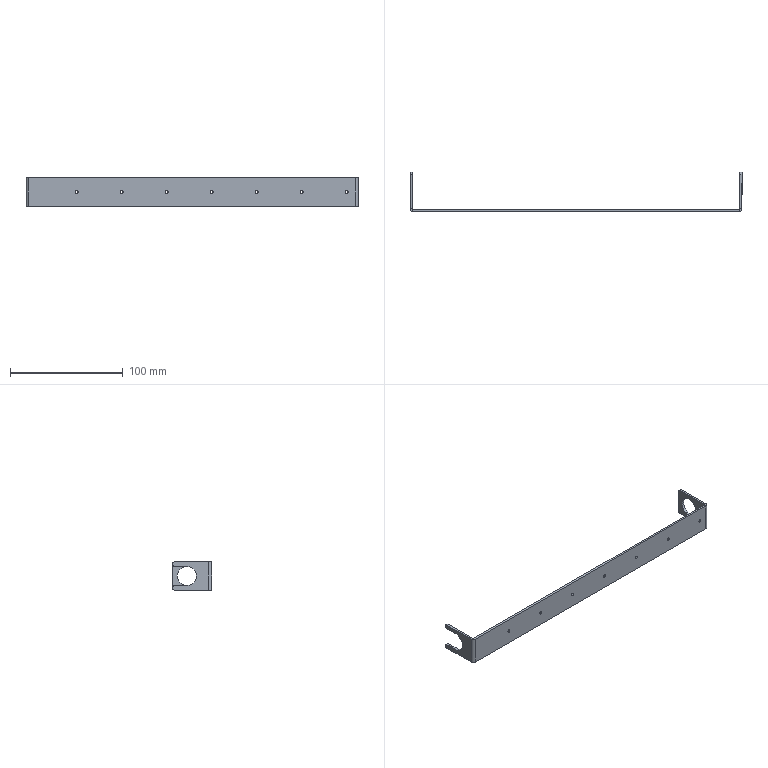Part | SolidWorks | features HoleWzd 2, ICE 2, EdgeFlange 1, Fillet 1, FlatPattern 1, LPattern 1, SMBaseFlange 1, SheetMetal 1 | 1 solid | 47 faces | box 295 x 35 x 25 mm | volume 16784 mm3 | cylinder 28 | plane 19 | commonest cylinder face diameters 2.5 x14 4 x6 17 x4 1 x2 5 x2
STEP:
#1=CARTESIAN_POINT('',(97.5,-2.,-1.25));
#2=VERTEX_POINT('',#1);
#3=CARTESIAN_POINT('',(97.5,-2.,1.25));
#4=VERTEX_POINT('',#3);
#5=CARTESIAN_POINT('',(97.5,-2.,0.));
#6=DIRECTION('',(0.,1.,0.));
#7=DIRECTION('',(0.,0.,1.));
#8=AXIS2_PLACEMENT_3D('',#5,#6,#7);
#9=CIRCLE('',#8,1.25);
#10=EDGE_CURVE('',#2,#4,#9,.T.);
#11=ORIENTED_EDGE('',*,*,#10,.F.);
#12=CARTESIAN_POINT('',(97.5,0.,-1.25));
#13=VERTEX_POINT('',#12);
#14=CARTESIAN_POINT('',(97.5,0.,-1.25));
#15=DIRECTION('',(0.,1.,0.));
#16=VECTOR('',#15,1000.);
#17=LINE('',#14,#16);
#18=EDGE_CURVE('',#2,#13,#17,.T.);
#19=ORIENTED_EDGE('',*,*,#18,.T.);
#20=CARTESIAN_POINT('',(97.5,0.,1.25));
#21=VERTEX_POINT('',#20);
#22=CARTESIAN_POINT('',(97.5,0.,0.));
#23=DIRECTION('',(0.,1.,0.));
#24=DIRECTION('',(0.,0.,1.));
#25=AXIS2_PLACEMENT_3D('',#22,#23,#24);
#26=CIRCLE('',#25,1.25);
#27=EDGE_CURVE('',#13,#21,#26,.T.);
#28=ORIENTED_EDGE('',*,*,#27,.T.);
#29=CARTESIAN_POINT('',(97.5,0.,1.25));
#30=DIRECTION('',(0.,1.,0.));
#31=VECTOR('',#30,1000.);
#32=LINE('',#29,#31);
#33=EDGE_CURVE('',#4,#21,#32,.T.);
#34=ORIENTED_EDGE('',*,*,#33,.F.);
#35=EDGE_LOOP('',(#11,#19,#28,#34));
#36=FACE_OUTER_BOUND('',#35,.T.);
#37=CARTESIAN_POINT('',(97.5,0.,0.));
#38=DIRECTION('',(0.,1.,0.));
#39=DIRECTION('',(0.,0.,1.));
#40=AXIS2_PLACEMENT_3D('',#37,#38,#39);
#41=CYLINDRICAL_SURFACE('',#40,1.25);
#42=ADVANCED_FACE('',(#36),#41,.F.);
#43=CARTESIAN_POINT('',(137.5,-2.,-1.25));
#44=VERTEX_POINT('',#43);
#45=CARTESIAN_POINT('',(137.5,-2.,1.25));
#46=VERTEX_POINT('',#45);
#47=CARTESIAN_POINT('',(137.5,-2.,0.));
#48=DIRECTION('',(0.,1.,0.));
#49=DIRECTION('',(0.,0.,1.));
#50=AXIS2_PLACEMENT_3D('',#47,#48,#49);
#51=CIRCLE('',#50,1.25);
#52=EDGE_CURVE('',#44,#46,#51,.T.);
#53=ORIENTED_EDGE('',*,*,#52,.F.);
#54=CARTESIAN_POINT('',(137.5,0.,-1.25));
#55=VERTEX_POINT('',#54);
#56=CARTESIAN_POINT('',(137.5,0.,-1.25));
#57=DIRECTION('',(0.,1.,0.));
#58=VECTOR('',#57,1000.);
#59=LINE('',#56,#58);
#60=EDGE_CURVE('',#44,#55,#59,.T.);
#61=ORIENTED_EDGE('',*,*,#60,.T.);
#62=CARTESIAN_POINT('',(137.5,0.,1.25));
#63=VERTEX_POINT('',#62);
#64=CARTESIAN_POINT('',(137.5,0.,0.));
#65=DIRECTION('',(0.,1.,0.));
#66=DIRECTION('',(0.,0.,1.));
#67=AXIS2_PLACEMENT_3D('',#64,#65,#66);
#68=CIRCLE('',#67,1.25);
#69=EDGE_CURVE('',#55,#63,#68,.T.);
#70=ORIENTED_EDGE('',*,*,#69,.T.);
#71=CARTESIAN_POINT('',(137.5,0.,1.25));
#72=DIRECTION('',(0.,1.,0.));
#73=VECTOR('',#72,1000.);
#74=LINE('',#71,#73);
#75=EDGE_CURVE('',#46,#63,#74,.T.);
#76=ORIENTED_EDGE('',*,*,#75,.F.);
#77=EDGE_LOOP('',(#53,#61,#70,#76));
#78=FACE_OUTER_BOUND('',#77,.T.);
#79=CARTESIAN_POINT('',(137.5,0.,0.));
#80=DIRECTION('',(0.,1.,0.));
#81=DIRECTION('',(0.,0.,1.));
#82=AXIS2_PLACEMENT_3D('',#79,#80,#81);
#83=CYLINDRICAL_SURFACE('',#82,1.25);
#84=ADVANCED_FACE('',(#78),#83,.F.);
#85=CARTESIAN_POINT('',(-145.5,20.,8.5));
#86=VERTEX_POINT('',#85);
#87=CARTESIAN_POINT('',(-145.5,11.5,0.));
#88=VERTEX_POINT('',#87);
#89=CARTESIAN_POINT('',(-145.5,20.,0.));
#90=DIRECTION('',(1.,0.,0.));
#91=DIRECTION('',(0.,1.,0.));
#92=AXIS2_PLACEMENT_3D('',#89,#90,#91);
#93=CIRCLE('',#92,8.5);
#94=EDGE_CURVE('',#86,#88,#93,.T.);
#95=ORIENTED_EDGE('',*,*,#94,.T.);
#96=CARTESIAN_POINT('',(-147.5,11.5,0.));
#97=VERTEX_POINT('',#96);
#98=CARTESIAN_POINT('',(-137.5,11.5,0.));
#99=DIRECTION('',(-1.,0.,0.));
#100=VECTOR('',#99,1000.);
#101=LINE('',#98,#100);
#102=EDGE_CURVE('',#88,#97,#101,.T.);
#103=ORIENTED_EDGE('',*,*,#102,.T.);
#104=CARTESIAN_POINT('',(-147.5,20.,8.5));
#105=VERTEX_POINT('',#104);
#106=CARTESIAN_POINT('',(-147.5,20.,0.));
#107=DIRECTION('',(-1.,0.,0.));
#108=DIRECTION('',(0.,-1.,0.));
#109=AXIS2_PLACEMENT_3D('',#106,#107,#108);
#110=CIRCLE('',#109,8.5);
#111=EDGE_CURVE('',#97,#105,#110,.T.);
#112=ORIENTED_EDGE('',*,*,#111,.T.);
#113=CARTESIAN_POINT('',(-137.5,20.,8.5));
#114=DIRECTION('',(-1.,0.,0.));
#115=VECTOR('',#114,1000.);
#116=LINE('',#113,#115);
#117=EDGE_CURVE('',#86,#105,#116,.T.);
#118=ORIENTED_EDGE('',*,*,#117,.F.);
#119=EDGE_LOOP('',(#95,#103,#112,#118));
#120=FACE_OUTER_BOUND('',#119,.T.);
#121=CARTESIAN_POINT('',(-137.5,20.,0.));
#122=DIRECTION('',(-1.,0.,0.));
#123=DIRECTION('',(0.,-1.,0.));
#124=AXIS2_PLACEMENT_3D('',#121,#122,#123);
#125=CYLINDRICAL_SURFACE('',#124,8.5);
#126=ADVANCED_FACE('',(#120),#125,.F.);
#127=CARTESIAN_POINT('',(145.5,28.5,0.));
#128=VERTEX_POINT('',#127);
#129=CARTESIAN_POINT('',(145.5,11.5,0.));
#130=VERTEX_POINT('',#129);
#131=CARTESIAN_POINT('',(145.5,20.,0.));
#132=DIRECTION('',(-1.,0.,0.));
#133=DIRECTION('',(0.,-1.,0.));
#134=AXIS2_PLACEMENT_3D('',#131,#132,#133);
#135=CIRCLE('',#134,8.5);
#136=EDGE_CURVE('',#128,#130,#135,.T.);
#137=ORIENTED_EDGE('',*,*,#136,.T.);
#138=CARTESIAN_POINT('',(147.5,11.5,0.));
#139=VERTEX_POINT('',#138);
#140=CARTESIAN_POINT('',(137.5,11.5,0.));
#141=DIRECTION('',(1.,0.,0.));
#142=VECTOR('',#141,1000.);
#143=LINE('',#140,#142);
#144=EDGE_CURVE('',#130,#139,#143,.T.);
#145=ORIENTED_EDGE('',*,*,#144,.T.);
#146=CARTESIAN_POINT('',(147.5,28.5,0.));
#147=VERTEX_POINT('',#146);
#148=CARTESIAN_POINT('',(147.5,20.,0.));
#149=DIRECTION('',(1.,0.,0.));
#150=DIRECTION('',(0.,1.,0.));
#151=AXIS2_PLACEMENT_3D('',#148,#149,#150);
#152=CIRCLE('',#151,8.5);
#153=EDGE_CURVE('',#139,#147,#152,.T.);
#154=ORIENTED_EDGE('',*,*,#153,.T.);
#155=CARTESIAN_POINT('',(137.5,28.5,0.));
#156=DIRECTION('',(1.,0.,0.));
#157=VECTOR('',#156,1000.);
#158=LINE('',#155,#157);
#159=EDGE_CURVE('',#128,#147,#158,.T.);
#160=ORIENTED_EDGE('',*,*,#159,.F.);
#161=EDGE_LOOP('',(#137,#145,#154,#160));
#162=FACE_OUTER_BOUND('',#161,.T.);
#163=CARTESIAN_POINT('',(137.5,20.,0.));
#164=DIRECTION('',(1.,0.,0.));
#165=DIRECTION('',(0.,1.,0.));
#166=AXIS2_PLACEMENT_3D('',#163,#164,#165);
#167=CYLINDRICAL_SURFACE('',#166,8.5);
#168=ADVANCED_FACE('',(#162),#167,.F.);
#169=CARTESIAN_POINT('',(57.5,-2.,-1.25));
#170=VERTEX_POINT('',#169);
#171=CARTESIAN_POINT('',(57.5,-2.,1.25));
#172=VERTEX_POINT('',#171);
#173=CARTESIAN_POINT('',(57.5,-2.,0.));
#174=DIRECTION('',(0.,1.,0.));
#175=DIRECTION('',(0.,0.,1.));
#176=AXIS2_PLACEMENT_3D('',#173,#174,#175);
#177=CIRCLE('',#176,1.25);
#178=EDGE_CURVE('',#170,#172,#177,.T.);
#179=ORIENTED_EDGE('',*,*,#178,.F.);
#180=CARTESIAN_POINT('',(57.5,0.,-1.25));
#181=VERTEX_POINT('',#180);
#182=CARTESIAN_POINT('',(57.5,0.,-1.25));
#183=DIRECTION('',(0.,1.,0.));
#184=VECTOR('',#183,1000.);
#185=LINE('',#182,#184);
#186=EDGE_CURVE('',#170,#181,#185,.T.);
#187=ORIENTED_EDGE('',*,*,#186,.T.);
#188=CARTESIAN_POINT('',(57.5,0.,1.25));
#189=VERTEX_POINT('',#188);
#190=CARTESIAN_POINT('',(57.5,0.,0.));
#191=DIRECTION('',(0.,1.,0.));
#192=DIRECTION('',(0.,0.,1.));
#193=AXIS2_PLACEMENT_3D('',#190,#191,#192);
#194=CIRCLE('',#193,1.25);
#195=EDGE_CURVE('',#181,#189,#194,.T.);
#196=ORIENTED_EDGE('',*,*,#195,.T.);
#197=CARTESIAN_POINT('',(57.5,0.,1.25));
#198=DIRECTION('',(0.,1.,0.));
#199=VECTOR('',#198,1000.);
#200=LINE('',#197,#199);
#201=EDGE_CURVE('',#172,#189,#200,.T.);
#202=ORIENTED_EDGE('',*,*,#201,.F.);
#203=EDGE_LOOP('',(#179,#187,#196,#202));
#204=FACE_OUTER_BOUND('',#203,.T.);
#205=CARTESIAN_POINT('',(57.5,0.,0.));
#206=DIRECTION('',(0.,1.,0.));
#207=DIRECTION('',(0.,0.,1.));
#208=AXIS2_PLACEMENT_3D('',#205,#206,#207);
#209=CYLINDRICAL_SURFACE('',#208,1.25);
#210=ADVANCED_FACE('',(#204),#209,.F.);
#211=CARTESIAN_POINT('',(17.5,-2.,-1.25));
#212=VERTEX_POINT('',#211);
#213=CARTESIAN_POINT('',(17.5,-2.,1.25));
#214=VERTEX_POINT('',#213);
#215=CARTESIAN_POINT('',(17.5,-2.,0.));
#216=DIRECTION('',(0.,1.,0.));
#217=DIRECTION('',(0.,0.,1.));
#218=AXIS2_PLACEMENT_3D('',#215,#216,#217);
#219=CIRCLE('',#218,1.25);
#220=EDGE_CURVE('',#212,#214,#219,.T.);
#221=ORIENTED_EDGE('',*,*,#220,.F.);
#222=CARTESIAN_POINT('',(17.5,0.,-1.25));
#223=VERTEX_POINT('',#222);
#224=CARTESIAN_POINT('',(17.5,0.,-1.25));
#225=DIRECTION('',(0.,1.,0.));
#226=VECTOR('',#225,1000.);
#227=LINE('',#224,#226);
#228=EDGE_CURVE('',#212,#223,#227,.T.);
#229=ORIENTED_EDGE('',*,*,#228,.T.);
#230=CARTESIAN_POINT('',(17.5,0.,1.25));
#231=VERTEX_POINT('',#230);
#232=CARTESIAN_POINT('',(17.5,0.,0.));
#233=DIRECTION('',(0.,1.,0.));
#234=DIRECTION('',(0.,0.,1.));
#235=AXIS2_PLACEMENT_3D('',#232,#233,#234);
#236=CIRCLE('',#235,1.25);
#237=EDGE_CURVE('',#223,#231,#236,.T.);
#238=ORIENTED_EDGE('',*,*,#237,.T.);
#239=CARTESIAN_POINT('',(17.5,0.,1.25));
#240=DIRECTION('',(0.,1.,0.));
#241=VECTOR('',#240,1000.);
#242=LINE('',#239,#241);
#243=EDGE_CURVE('',#214,#231,#242,.T.);
#244=ORIENTED_EDGE('',*,*,#243,.F.);
#245=EDGE_LOOP('',(#221,#229,#238,#244));
#246=FACE_OUTER_BOUND('',#245,.T.);
#247=CARTESIAN_POINT('',(17.5,0.,0.));
#248=DIRECTION('',(0.,1.,0.));
#249=DIRECTION('',(0.,0.,1.));
#250=AXIS2_PLACEMENT_3D('',#247,#248,#249);
#251=CYLINDRICAL_SURFACE('',#250,1.25);
#252=ADVANCED_FACE('',(#246),#251,.F.);
#253=CARTESIAN_POINT('',(-22.5,-2.,-1.25));
#254=VERTEX_POINT('',#253);
#255=CARTESIAN_POINT('',(-22.5,-2.,1.25));
#256=VERTEX_POINT('',#255);
#257=CARTESIAN_POINT('',(-22.5,-2.,0.));
#258=DIRECTION('',(0.,1.,0.));
#259=DIRECTION('',(0.,0.,1.));
#260=AXIS2_PLACEMENT_3D('',#257,#258,#259);
#261=CIRCLE('',#260,1.25);
#262=EDGE_CURVE('',#254,#256,#261,.T.);
#263=ORIENTED_EDGE('',*,*,#262,.F.);
#264=CARTESIAN_POINT('',(-22.5,0.,-1.25));
#265=VERTEX_POINT('',#264);
#266=CARTESIAN_POINT('',(-22.5,0.,-1.25));
#267=DIRECTION('',(0.,1.,0.));
#268=VECTOR('',#267,1000.);
#269=LINE('',#266,#268);
#270=EDGE_CURVE('',#254,#265,#269,.T.);
#271=ORIENTED_EDGE('',*,*,#270,.T.);
#272=CARTESIAN_POINT('',(-22.5,0.,1.25));
#273=VERTEX_POINT('',#272);
#274=CARTESIAN_POINT('',(-22.5,0.,0.));
#275=DIRECTION('',(0.,1.,0.));
#276=DIRECTION('',(0.,0.,1.));
#277=AXIS2_PLACEMENT_3D('',#274,#275,#276);
#278=CIRCLE('',#277,1.25);
#279=EDGE_CURVE('',#265,#273,#278,.T.);
#280=ORIENTED_EDGE('',*,*,#279,.T.);
#281=CARTESIAN_POINT('',(-22.5,0.,1.25));
#282=DIRECTION('',(0.,1.,0.));
#283=VECTOR('',#282,1000.);
#284=LINE('',#281,#283);
#285=EDGE_CURVE('',#256,#273,#284,.T.);
#286=ORIENTED_EDGE('',*,*,#285,.F.);
#287=EDGE_LOOP('',(#263,#271,#280,#286));
#288=FACE_OUTER_BOUND('',#287,.T.);
#289=CARTESIAN_POINT('',(-22.5,0.,0.));
#290=DIRECTION('',(0.,1.,0.));
#291=DIRECTION('',(0.,0.,1.));
#292=AXIS2_PLACEMENT_3D('',#289,#290,#291);
#293=CYLINDRICAL_SURFACE('',#292,1.25);
#294=ADVANCED_FACE('',(#288),#293,.F.);
#295=CARTESIAN_POINT('',(-62.5,-2.,-1.25));
#296=VERTEX_POINT('',#295);
#297=CARTESIAN_POINT('',(-62.5,-2.,1.25));
#298=VERTEX_POINT('',#297);
#299=CARTESIAN_POINT('',(-62.5,-2.,0.));
#300=DIRECTION('',(0.,1.,0.));
#301=DIRECTION('',(0.,0.,1.));
#302=AXIS2_PLACEMENT_3D('',#299,#300,#301);
#303=CIRCLE('',#302,1.25);
#304=EDGE_CURVE('',#296,#298,#303,.T.);
#305=ORIENTED_EDGE('',*,*,#304,.F.);
#306=CARTESIAN_POINT('',(-62.5,0.,-1.25));
#307=VERTEX_POINT('',#306);
#308=CARTESIAN_POINT('',(-62.5,0.,-1.25));
#309=DIRECTION('',(0.,1.,0.));
#310=VECTOR('',#309,1000.);
#311=LINE('',#308,#310);
#312=EDGE_CURVE('',#296,#307,#311,.T.);
#313=ORIENTED_EDGE('',*,*,#312,.T.);
#314=CARTESIAN_POINT('',(-62.5,0.,1.25));
#315=VERTEX_POINT('',#314);
#316=CARTESIAN_POINT('',(-62.5,0.,0.));
#317=DIRECTION('',(0.,1.,0.));
#318=DIRECTION('',(0.,0.,1.));
#319=AXIS2_PLACEMENT_3D('',#316,#317,#318);
#320=CIRCLE('',#319,1.25);
#321=EDGE_CURVE('',#307,#315,#320,.T.);
#322=ORIENTED_EDGE('',*,*,#321,.T.);
#323=CARTESIAN_POINT('',(-62.5,0.,1.25));
#324=DIRECTION('',(0.,1.,0.));
#325=VECTOR('',#324,1000.);
#326=LINE('',#323,#325);
#327=EDGE_CURVE('',#298,#315,#326,.T.);
#328=ORIENTED_EDGE('',*,*,#327,.F.);
#329=EDGE_LOOP('',(#305,#313,#322,#328));
#330=FACE_OUTER_BOUND('',#329,.T.);
#331=CARTESIAN_POINT('',(-62.5,0.,0.));
#332=DIRECTION('',(0.,1.,0.));
#333=DIRECTION('',(0.,0.,1.));
#334=AXIS2_PLACEMENT_3D('',#331,#332,#333);
#335=CYLINDRICAL_SURFACE('',#334,1.25);
#336=ADVANCED_FACE('',(#330),#335,.F.);
#337=CARTESIAN_POINT('',(-102.5,-2.,-1.25));
#338=VERTEX_POINT('',#337);
#339=CARTESIAN_POINT('',(-102.5,-2.,1.25));
#340=VERTEX_POINT('',#339);
#341=CARTESIAN_POINT('',(-102.5,-2.,0.));
#342=DIRECTION('',(0.,1.,0.));
#343=DIRECTION('',(0.,0.,1.));
#344=AXIS2_PLACEMENT_3D('',#341,#342,#343);
#345=CIRCLE('',#344,1.25);
#346=EDGE_CURVE('',#338,#340,#345,.T.);
#347=ORIENTED_EDGE('',*,*,#346,.F.);
#348=CARTESIAN_POINT('',(-102.5,0.,-1.25));
#349=VERTEX_POINT('',#348);
#350=CARTESIAN_POINT('',(-102.5,0.,-1.25));
#351=DIRECTION('',(0.,1.,0.));
#352=VECTOR('',#351,1000.);
#353=LINE('',#350,#352);
#354=EDGE_CURVE('',#338,#349,#353,.T.);
#355=ORIENTED_EDGE('',*,*,#354,.T.);
#356=CARTESIAN_POINT('',(-102.5,0.,1.25));
#357=VERTEX_POINT('',#356);
#358=CARTESIAN_POINT('',(-102.5,0.,0.));
#359=DIRECTION('',(0.,1.,0.));
#360=DIRECTION('',(0.,0.,1.));
#361=AXIS2_PLACEMENT_3D('',#358,#359,#360);
#362=CIRCLE('',#361,1.25);
#363=EDGE_CURVE('',#349,#357,#362,.T.);
#364=ORIENTED_EDGE('',*,*,#363,.T.);
#365=CARTESIAN_POINT('',(-102.5,0.,1.25));
#366=DIRECTION('',(0.,1.,0.));
#367=VECTOR('',#366,1000.);
#368=LINE('',#365,#367);
#369=EDGE_CURVE('',#340,#357,#368,.T.);
#370=ORIENTED_EDGE('',*,*,#369,.F.);
#371=EDGE_LOOP('',(#347,#355,#364,#370));
#372=FACE_OUTER_BOUND('',#371,.T.);
#373=CARTESIAN_POINT('',(-102.5,0.,0.));
#374=DIRECTION('',(0.,1.,0.));
#375=DIRECTION('',(0.,0.,1.));
#376=AXIS2_PLACEMENT_3D('',#373,#374,#375);
#377=CYLINDRICAL_SURFACE('',#376,1.25);
#378=ADVANCED_FACE('',(#372),#377,.F.);
#379=ORIENTED_EDGE('',*,*,#354,.F.);
#380=CARTESIAN_POINT('',(-102.5,-2.,0.));
#381=DIRECTION('',(0.,1.,0.));
#382=DIRECTION('',(0.,0.,1.));
#383=AXIS2_PLACEMENT_3D('',#380,#381,#382);
#384=CIRCLE('',#383,1.25);
#385=EDGE_CURVE('',#340,#338,#384,.T.);
#386=ORIENTED_EDGE('',*,*,#385,.F.);
#387=ORIENTED_EDGE('',*,*,#369,.T.);
#388=CARTESIAN_POINT('',(-102.5,0.,0.));
#389=DIRECTION('',(0.,1.,0.));
#390=DIRECTION('',(0.,0.,1.));
#391=AXIS2_PLACEMENT_3D('',#388,#389,#390);
#392=CIRCLE('',#391,1.25);
#393=EDGE_CURVE('',#357,#349,#392,.T.);
#394=ORIENTED_EDGE('',*,*,#393,.T.);
#395=EDGE_LOOP('',(#379,#386,#387,#394));
#396=FACE_OUTER_BOUND('',#395,.T.);
#397=CARTESIAN_POINT('',(-102.5,0.,0.));
#398=DIRECTION('',(0.,1.,0.));
#399=DIRECTION('',(0.,0.,1.));
#400=AXIS2_PLACEMENT_3D('',#397,#398,#399);
#401=CYLINDRICAL_SURFACE('',#400,1.25);
#402=ADVANCED_FACE('',(#396),#401,.F.);
#403=ORIENTED_EDGE('',*,*,#312,.F.);
#404=CARTESIAN_POINT('',(-62.5,-2.,0.));
#405=DIRECTION('',(0.,1.,0.));
#406=DIRECTION('',(0.,0.,1.));
#407=AXIS2_PLACEMENT_3D('',#404,#405,#406);
#408=CIRCLE('',#407,1.25);
#409=EDGE_CURVE('',#298,#296,#408,.T.);
#410=ORIENTED_EDGE('',*,*,#409,.F.);
#411=ORIENTED_EDGE('',*,*,#327,.T.);
#412=CARTESIAN_POINT('',(-62.5,0.,0.));
#413=DIRECTION('',(0.,1.,0.));
#414=DIRECTION('',(0.,0.,1.));
#415=AXIS2_PLACEMENT_3D('',#412,#413,#414);
#416=CIRCLE('',#415,1.25);
#417=EDGE_CURVE('',#315,#307,#416,.T.);
#418=ORIENTED_EDGE('',*,*,#417,.T.);
#419=EDGE_LOOP('',(#403,#410,#411,#418));
#420=FACE_OUTER_BOUND('',#419,.T.);
#421=CARTESIAN_POINT('',(-62.5,0.,0.));
#422=DIRECTION('',(0.,1.,0.));
#423=DIRECTION('',(0.,0.,1.));
#424=AXIS2_PLACEMENT_3D('',#421,#422,#423);
#425=CYLINDRICAL_SURFACE('',#424,1.25);
#426=ADVANCED_FACE('',(#420),#425,.F.);
#427=ORIENTED_EDGE('',*,*,#270,.F.);
#428=CARTESIAN_POINT('',(-22.5,-2.,0.));
#429=DIRECTION('',(0.,1.,0.));
#430=DIRECTION('',(0.,0.,1.));
#431=AXIS2_PLACEMENT_3D('',#428,#429,#430);
#432=CIRCLE('',#431,1.25);
#433=EDGE_CURVE('',#256,#254,#432,.T.);
#434=ORIENTED_EDGE('',*,*,#433,.F.);
#435=ORIENTED_EDGE('',*,*,#285,.T.);
#436=CARTESIAN_POINT('',(-22.5,0.,0.));
#437=DIRECTION('',(0.,1.,0.));
#438=DIRECTION('',(0.,0.,1.));
#439=AXIS2_PLACEMENT_3D('',#436,#437,#438);
#440=CIRCLE('',#439,1.25);
#441=EDGE_CURVE('',#273,#265,#440,.T.);
#442=ORIENTED_EDGE('',*,*,#441,.T.);
#443=EDGE_LOOP('',(#427,#434,#435,#442));
#444=FACE_OUTER_BOUND('',#443,.T.);
#445=CARTESIAN_POINT('',(-22.5,0.,0.));
#446=DIRECTION('',(0.,1.,0.));
#447=DIRECTION('',(0.,0.,1.));
#448=AXIS2_PLACEMENT_3D('',#445,#446,#447);
#449=CYLINDRICAL_SURFACE('',#448,1.25);
#450=ADVANCED_FACE('',(#444),#449,.F.);
#451=ORIENTED_EDGE('',*,*,#228,.F.);
#452=CARTESIAN_POINT('',(17.5,-2.,0.));
#453=DIRECTION('',(0.,1.,0.));
#454=DIRECTION('',(0.,0.,1.));
#455=AXIS2_PLACEMENT_3D('',#452,#453,#454);
#456=CIRCLE('',#455,1.25);
#457=EDGE_CURVE('',#214,#212,#456,.T.);
#458=ORIENTED_EDGE('',*,*,#457,.F.);
#459=ORIENTED_EDGE('',*,*,#243,.T.);
#460=CARTESIAN_POINT('',(17.5,0.,0.));
#461=DIRECTION('',(0.,1.,0.));
#462=DIRECTION('',(0.,0.,1.));
#463=AXIS2_PLACEMENT_3D('',#460,#461,#462);
#464=CIRCLE('',#463,1.25);
#465=EDGE_CURVE('',#231,#223,#464,.T.);
#466=ORIENTED_EDGE('',*,*,#465,.T.);
#467=EDGE_LOOP('',(#451,#458,#459,#466));
#468=FACE_OUTER_BOUND('',#467,.T.);
#469=CARTESIAN_POINT('',(17.5,0.,0.));
#470=DIRECTION('',(0.,1.,0.));
#471=DIRECTION('',(0.,0.,1.));
#472=AXIS2_PLACEMENT_3D('',#469,#470,#471);
#473=CYLINDRICAL_SURFACE('',#472,1.25);
#474=ADVANCED_FACE('',(#468),#473,.F.);
#475=ORIENTED_EDGE('',*,*,#186,.F.);
#476=CARTESIAN_POINT('',(57.5,-2.,0.));
#477=DIRECTION('',(0.,1.,0.));
#478=DIRECTION('',(0.,0.,1.));
#479=AXIS2_PLACEMENT_3D('',#476,#477,#478);
#480=CIRCLE('',#479,1.25);
#481=EDGE_CURVE('',#172,#170,#480,.T.);
#482=ORIENTED_EDGE('',*,*,#481,.F.);
#483=ORIENTED_EDGE('',*,*,#201,.T.);
#484=CARTESIAN_POINT('',(57.5,0.,0.));
#485=DIRECTION('',(0.,1.,0.));
#486=DIRECTION('',(0.,0.,1.));
#487=AXIS2_PLACEMENT_3D('',#484,#485,#486);
#488=CIRCLE('',#487,1.25);
#489=EDGE_CURVE('',#189,#181,#488,.T.);
#490=ORIENTED_EDGE('',*,*,#489,.T.);
#491=EDGE_LOOP('',(#475,#482,#483,#490));
#492=FACE_OUTER_BOUND('',#491,.T.);
#493=CARTESIAN_POINT('',(57.5,0.,0.));
#494=DIRECTION('',(0.,1.,0.));
#495=DIRECTION('',(0.,0.,1.));
#496=AXIS2_PLACEMENT_3D('',#493,#494,#495);
#497=CYLINDRICAL_SURFACE('',#496,1.25);
#498=ADVANCED_FACE('',(#492),#497,.F.);
#499=CARTESIAN_POINT('',(97.5,-2.,0.));
#500=DIRECTION('',(0.,1.,0.));
#501=DIRECTION('',(0.,0.,1.));
#502=AXIS2_PLACEMENT_3D('',#499,#500,#501);
#503=CIRCLE('',#502,1.25);
#504=EDGE_CURVE('',#4,#2,#503,.T.);
#505=ORIENTED_EDGE('',*,*,#504,.T.);
#506=ORIENTED_EDGE('',*,*,#10,.T.);
#507=EDGE_LOOP('',(#505,#506));
#508=FACE_BOUND('',#507,.T.);
#509=CARTESIAN_POINT('',(137.5,-2.,0.));
#510=DIRECTION('',(0.,1.,0.));
#511=DIRECTION('',(0.,0.,1.));
#512=AXIS2_PLACEMENT_3D('',#509,#510,#511);
#513=CIRCLE('',#512,1.25);
#514=EDGE_CURVE('',#46,#44,#513,.T.);
#515=ORIENTED_EDGE('',*,*,#514,.T.);
#516=ORIENTED_EDGE('',*,*,#52,.T.);
#517=EDGE_LOOP('',(#515,#516));
#518=FACE_BOUND('',#517,.T.);
#519=CARTESIAN_POINT('',(145.,-2.,-12.5));
#520=VERTEX_POINT('',#519);
#521=CARTESIAN_POINT('',(145.,-2.,12.5));
#522=VERTEX_POINT('',#521);
#523=CARTESIAN_POINT('',(145.,-2.,-12.5));
#524=DIRECTION('',(0.,0.,1.));
#525=VECTOR('',#524,1000.);
#526=LINE('',#523,#525);
#527=EDGE_CURVE('',#520,#522,#526,.T.);
#528=ORIENTED_EDGE('',*,*,#527,.T.);
#529=CARTESIAN_POINT('',(-145.,-2.,12.5));
#530=VERTEX_POINT('',#529);
#531=CARTESIAN_POINT('',(147.5,-2.,12.5));
#532=DIRECTION('',(1.,0.,0.));
#533=VECTOR('',#532,1000.);
#534=LINE('',#531,#533);
#535=EDGE_CURVE('',#530,#522,#534,.T.);
#536=ORIENTED_EDGE('',*,*,#535,.F.);
#537=CARTESIAN_POINT('',(-145.,-2.,-12.5));
#538=VERTEX_POINT('',#537);
#539=CARTESIAN_POINT('',(-145.,-2.,12.5));
#540=DIRECTION('',(0.,0.,-1.));
#541=VECTOR('',#540,1000.);
#542=LINE('',#539,#541);
#543=EDGE_CURVE('',#530,#538,#542,.T.);
#544=ORIENTED_EDGE('',*,*,#543,.T.);
#545=CARTESIAN_POINT('',(147.5,-2.,-12.5));
#546=DIRECTION('',(-1.,0.,0.));
#547=VECTOR('',#546,1000.);
#548=LINE('',#545,#547);
#549=EDGE_CURVE('',#520,#538,#548,.T.);
#550=ORIENTED_EDGE('',*,*,#549,.F.);
#551=EDGE_LOOP('',(#528,#536,#544,#550));
#552=FACE_OUTER_BOUND('',#551,.T.);
#553=ORIENTED_EDGE('',*,*,#481,.T.);
#554=ORIENTED_EDGE('',*,*,#178,.T.);
#555=EDGE_LOOP('',(#553,#554));
#556=FACE_BOUND('',#555,.T.);
#557=ORIENTED_EDGE('',*,*,#457,.T.);
#558=ORIENTED_EDGE('',*,*,#220,.T.);
#559=EDGE_LOOP('',(#557,#558));
#560=FACE_BOUND('',#559,.T.);
#561=ORIENTED_EDGE('',*,*,#433,.T.);
#562=ORIENTED_EDGE('',*,*,#262,.T.);
#563=EDGE_LOOP('',(#561,#562));
#564=FACE_BOUND('',#563,.T.);
#565=ORIENTED_EDGE('',*,*,#409,.T.);
#566=ORIENTED_EDGE('',*,*,#304,.T.);
#567=EDGE_LOOP('',(#565,#566));
#568=FACE_BOUND('',#567,.T.);
#569=ORIENTED_EDGE('',*,*,#385,.T.);
#570=ORIENTED_EDGE('',*,*,#346,.T.);
#571=EDGE_LOOP('',(#569,#570));
#572=FACE_BOUND('',#571,.T.);
#573=CARTESIAN_POINT('',(0.,-2.,0.));
#574=DIRECTION('',(0.,1.,0.));
#575=DIRECTION('',(0.,0.,1.));
#576=AXIS2_PLACEMENT_3D('',#573,#574,#575);
#577=PLANE('',#576);
#578=ADVANCED_FACE('',(#508,#518,#552,#556,#560,#564,#568,#572),#577,.F.);
#579=CARTESIAN_POINT('',(97.5,0.,0.));
#580=DIRECTION('',(0.,1.,0.));
#581=DIRECTION('',(0.,0.,1.));
#582=AXIS2_PLACEMENT_3D('',#579,#580,#581);
#583=CIRCLE('',#582,1.25);
#584=EDGE_CURVE('',#21,#13,#583,.T.);
#585=ORIENTED_EDGE('',*,*,#584,.F.);
#586=ORIENTED_EDGE('',*,*,#27,.F.);
#587=EDGE_LOOP('',(#585,#586));
#588=FACE_BOUND('',#587,.T.);
#589=CARTESIAN_POINT('',(137.5,0.,0.));
#590=DIRECTION('',(0.,1.,0.));
#591=DIRECTION('',(0.,0.,1.));
#592=AXIS2_PLACEMENT_3D('',#589,#590,#591);
#593=CIRCLE('',#592,1.25);
#594=EDGE_CURVE('',#63,#55,#593,.T.);
#595=ORIENTED_EDGE('',*,*,#594,.F.);
#596=ORIENTED_EDGE('',*,*,#69,.F.);
#597=EDGE_LOOP('',(#595,#596));
#598=FACE_BOUND('',#597,.T.);
#599=CARTESIAN_POINT('',(-145.,0.,12.5));
#600=VERTEX_POINT('',#599);
#601=CARTESIAN_POINT('',(145.,0.,12.5));
#602=VERTEX_POINT('',#601);
#603=CARTESIAN_POINT('',(147.5,0.,12.5));
#604=DIRECTION('',(1.,0.,0.));
#605=VECTOR('',#604,1000.);
#606=LINE('',#603,#605);
#607=EDGE_CURVE('',#600,#602,#606,.T.);
#608=ORIENTED_EDGE('',*,*,#607,.T.);
#609=CARTESIAN_POINT('',(145.,0.,-12.5));
#610=VERTEX_POINT('',#609);
#611=CARTESIAN_POINT('',(145.,0.,-12.5));
#612=DIRECTION('',(0.,0.,1.));
#613=VECTOR('',#612,1000.);
#614=LINE('',#611,#613);
#615=EDGE_CURVE('',#610,#602,#614,.T.);
#616=ORIENTED_EDGE('',*,*,#615,.F.);
#617=CARTESIAN_POINT('',(-145.,0.,-12.5));
#618=VERTEX_POINT('',#617);
#619=CARTESIAN_POINT('',(147.5,0.,-12.5));
#620=DIRECTION('',(-1.,0.,0.));
#621=VECTOR('',#620,1000.);
#622=LINE('',#619,#621);
#623=EDGE_CURVE('',#610,#618,#622,.T.);
#624=ORIENTED_EDGE('',*,*,#623,.T.);
#625=CARTESIAN_POINT('',(-145.,0.,12.5));
#626=DIRECTION('',(0.,0.,-1.));
#627=VECTOR('',#626,1000.);
#628=LINE('',#625,#627);
#629=EDGE_CURVE('',#600,#618,#628,.T.);
#630=ORIENTED_EDGE('',*,*,#629,.F.);
#631=EDGE_LOOP('',(#608,#616,#624,#630));
#632=FACE_OUTER_BOUND('',#631,.T.);
#633=ORIENTED_EDGE('',*,*,#489,.F.);
#634=ORIENTED_EDGE('',*,*,#195,.F.);
#635=EDGE_LOOP('',(#633,#634));
#636=FACE_BOUND('',#635,.T.);
#637=ORIENTED_EDGE('',*,*,#465,.F.);
#638=ORIENTED_EDGE('',*,*,#237,.F.);
#639=EDGE_LOOP('',(#637,#638));
#640=FACE_BOUND('',#639,.T.);
#641=ORIENTED_EDGE('',*,*,#441,.F.);
#642=ORIENTED_EDGE('',*,*,#279,.F.);
#643=EDGE_LOOP('',(#641,#642));
#644=FACE_BOUND('',#643,.T.);
#645=ORIENTED_EDGE('',*,*,#417,.F.);
#646=ORIENTED_EDGE('',*,*,#321,.F.);
#647=EDGE_LOOP('',(#645,#646));
#648=FACE_BOUND('',#647,.T.);
#649=ORIENTED_EDGE('',*,*,#393,.F.);
#650=ORIENTED_EDGE('',*,*,#363,.F.);
#651=EDGE_LOOP('',(#649,#650));
#652=FACE_BOUND('',#651,.T.);
#653=CARTESIAN_POINT('',(0.,0.,0.));
#654=DIRECTION('',(0.,1.,0.));
#655=DIRECTION('',(0.,0.,1.));
#656=AXIS2_PLACEMENT_3D('',#653,#654,#655);
#657=PLANE('',#656);
#658=ADVANCED_FACE('',(#588,#598,#632,#636,#640,#644,#648,#652),#657,.T.);
#659=ORIENTED_EDGE('',*,*,#623,.F.);
#660=CARTESIAN_POINT('',(145.,0.,-12.5));
#661=DIRECTION('',(0.,-1.,0.));
#662=VECTOR('',#661,1000.);
#663=LINE('',#660,#662);
#664=EDGE_CURVE('',#610,#520,#663,.T.);
#665=ORIENTED_EDGE('',*,*,#664,.T.);
#666=ORIENTED_EDGE('',*,*,#549,.T.);
#667=CARTESIAN_POINT('',(-145.,0.,-12.5));
#668=DIRECTION('',(0.,-1.,0.));
#669=VECTOR('',#668,1000.);
#670=LINE('',#667,#669);
#671=EDGE_CURVE('',#618,#538,#670,.T.);
#672=ORIENTED_EDGE('',*,*,#671,.F.);
#673=EDGE_LOOP('',(#659,#665,#666,#672));
#674=FACE_OUTER_BOUND('',#673,.T.);
#675=CARTESIAN_POINT('',(147.5,-2.,-12.5));
#676=DIRECTION('',(0.,0.,-1.));
#677=DIRECTION('',(-1.,0.,0.));
#678=AXIS2_PLACEMENT_3D('',#675,#676,#677);
#679=PLANE('',#678);
#680=ADVANCED_FACE('',(#674),#679,.T.);
#681=CARTESIAN_POINT('',(145.,0.,12.5));
#682=DIRECTION('',(0.,-1.,0.));
#683=VECTOR('',#682,1000.);
#684=LINE('',#681,#683);
#685=EDGE_CURVE('',#602,#522,#684,.T.);
#686=ORIENTED_EDGE('',*,*,#685,.F.);
#687=ORIENTED_EDGE('',*,*,#607,.F.);
#688=CARTESIAN_POINT('',(-145.,0.,12.5));
#689=DIRECTION('',(0.,-1.,0.));
#690=VECTOR('',#689,1000.);
#691=LINE('',#688,#690);
#692=EDGE_CURVE('',#600,#530,#691,.T.);
#693=ORIENTED_EDGE('',*,*,#692,.T.);
#694=ORIENTED_EDGE('',*,*,#535,.T.);
#695=EDGE_LOOP('',(#686,#687,#693,#694));
#696=FACE_OUTER_BOUND('',#695,.T.);
#697=CARTESIAN_POINT('',(147.5,-2.,12.5));
#698=DIRECTION('',(0.,0.,1.));
#699=DIRECTION('',(1.,0.,0.));
#700=AXIS2_PLACEMENT_3D('',#697,#698,#699);
#701=PLANE('',#700);
#702=ADVANCED_FACE('',(#696),#701,.T.);
#703=CARTESIAN_POINT('',(-145.5,0.5,-12.5));
#704=VERTEX_POINT('',#703);
#705=CARTESIAN_POINT('',(-147.5,0.5,-12.5));
#706=VERTEX_POINT('',#705);
#707=CARTESIAN_POINT('',(-147.5,0.5,-12.5));
#708=DIRECTION('',(-1.,0.,0.));
#709=VECTOR('',#708,1000.);
#710=LINE('',#707,#709);
#711=EDGE_CURVE('',#704,#706,#710,.T.);
#712=ORIENTED_EDGE('',*,*,#711,.F.);
#713=CARTESIAN_POINT('',(-145.,0.5,-12.5));
#714=DIRECTION('',(0.,0.,-1.));
#715=DIRECTION('',(1.,0.,0.));
#716=AXIS2_PLACEMENT_3D('',#713,#714,#715);
#717=CIRCLE('',#716,0.5);
#718=EDGE_CURVE('',#618,#704,#717,.T.);
#719=ORIENTED_EDGE('',*,*,#718,.F.);
#720=ORIENTED_EDGE('',*,*,#671,.T.);
#721=CARTESIAN_POINT('',(-145.,0.5,-12.5));
#722=DIRECTION('',(0.,0.,-1.));
#723=DIRECTION('',(1.,0.,0.));
#724=AXIS2_PLACEMENT_3D('',#721,#722,#723);
#725=CIRCLE('',#724,2.5);
#726=EDGE_CURVE('',#538,#706,#725,.T.);
#727=ORIENTED_EDGE('',*,*,#726,.T.);
#728=EDGE_LOOP('',(#712,#719,#720,#727));
#729=FACE_OUTER_BOUND('',#728,.T.);
#730=CARTESIAN_POINT('',(-145.,0.5,-12.5));
#731=DIRECTION('',(0.,0.,-1.));
#732=DIRECTION('',(-1.,0.,0.));
#733=AXIS2_PLACEMENT_3D('',#730,#731,#732);
#734=PLANE('',#733);
#735=ADVANCED_FACE('',(#729),#734,.T.);
#736=CARTESIAN_POINT('',(-145.5,0.5,12.5));
#737=VERTEX_POINT('',#736);
#738=CARTESIAN_POINT('',(-145.,0.5,12.5));
#739=DIRECTION('',(0.,0.,1.));
#740=DIRECTION('',(1.,0.,0.));
#741=AXIS2_PLACEMENT_3D('',#738,#739,#740);
#742=CIRCLE('',#741,0.5);
#743=EDGE_CURVE('',#737,#600,#742,.T.);
#744=ORIENTED_EDGE('',*,*,#743,.F.);
#745=CARTESIAN_POINT('',(-147.5,0.5,12.5));
#746=VERTEX_POINT('',#745);
#747=CARTESIAN_POINT('',(-145.5,0.5,12.5));
#748=DIRECTION('',(-1.,0.,0.));
#749=VECTOR('',#748,1000.);
#750=LINE('',#747,#749);
#751=EDGE_CURVE('',#737,#746,#750,.T.);
#752=ORIENTED_EDGE('',*,*,#751,.T.);
#753=CARTESIAN_POINT('',(-145.,0.5,12.5));
#754=DIRECTION('',(0.,0.,1.));
#755=DIRECTION('',(1.,0.,0.));
#756=AXIS2_PLACEMENT_3D('',#753,#754,#755);
#757=CIRCLE('',#756,2.5);
#758=EDGE_CURVE('',#746,#530,#757,.T.);
#759=ORIENTED_EDGE('',*,*,#758,.T.);
#760=ORIENTED_EDGE('',*,*,#692,.F.);
#761=EDGE_LOOP('',(#744,#752,#759,#760));
#762=FACE_OUTER_BOUND('',#761,.T.);
#763=CARTESIAN_POINT('',(-145.,0.5,12.5));
#764=DIRECTION('',(0.,0.,-1.));
#765=DIRECTION('',(-1.,0.,0.));
#766=AXIS2_PLACEMENT_3D('',#763,#764,#765);
#767=PLANE('',#766);
#768=ADVANCED_FACE('',(#762),#767,.F.);
#769=ORIENTED_EDGE('',*,*,#543,.F.);
#770=ORIENTED_EDGE('',*,*,#758,.F.);
#771=CARTESIAN_POINT('',(-147.5,0.5,-12.5));
#772=DIRECTION('',(0.,0.,-1.));
#773=VECTOR('',#772,1000.);
#774=LINE('',#771,#773);
#775=EDGE_CURVE('',#746,#706,#774,.T.);
#776=ORIENTED_EDGE('',*,*,#775,.T.);
#777=ORIENTED_EDGE('',*,*,#726,.F.);
#778=EDGE_LOOP('',(#769,#770,#776,#777));
#779=FACE_OUTER_BOUND('',#778,.T.);
#780=CARTESIAN_POINT('',(-145.,0.5,12.5));
#781=DIRECTION('',(0.,0.,1.));
#782=DIRECTION('',(-1.,0.,0.));
#783=AXIS2_PLACEMENT_3D('',#780,#781,#782);
#784=CYLINDRICAL_SURFACE('',#783,2.5);
#785=ADVANCED_FACE('',(#779),#784,.T.);
#786=ORIENTED_EDGE('',*,*,#629,.T.);
#787=ORIENTED_EDGE('',*,*,#718,.T.);
#788=CARTESIAN_POINT('',(-145.5,0.5,-12.5));
#789=DIRECTION('',(0.,0.,1.));
#790=VECTOR('',#789,1000.);
#791=LINE('',#788,#790);
#792=EDGE_CURVE('',#704,#737,#791,.T.);
#793=ORIENTED_EDGE('',*,*,#792,.T.);
#794=ORIENTED_EDGE('',*,*,#743,.T.);
#795=EDGE_LOOP('',(#786,#787,#793,#794));
#796=FACE_OUTER_BOUND('',#795,.T.);
#797=CARTESIAN_POINT('',(-145.,0.5,12.5));
#798=DIRECTION('',(0.,0.,1.));
#799=DIRECTION('',(-1.,0.,0.));
#800=AXIS2_PLACEMENT_3D('',#797,#798,#799);
#801=CYLINDRICAL_SURFACE('',#800,0.5);
#802=ADVANCED_FACE('',(#796),#801,.F.);
#803=CARTESIAN_POINT('',(-147.5,31.,-12.5));
#804=VERTEX_POINT('',#803);
#805=CARTESIAN_POINT('',(-147.5,0.,-12.5));
#806=DIRECTION('',(0.,-1.,0.));
#807=VECTOR('',#806,1000.);
#808=LINE('',#805,#807);
#809=EDGE_CURVE('',#804,#706,#808,.T.);
#810=ORIENTED_EDGE('',*,*,#809,.F.);
#811=CARTESIAN_POINT('',(-145.5,31.,-12.5));
#812=VERTEX_POINT('',#811);
#813=CARTESIAN_POINT('',(-147.5,31.,-12.5));
#814=DIRECTION('',(1.,0.,0.));
#815=VECTOR('',#814,1000.);
#816=LINE('',#813,#815);
#817=EDGE_CURVE('',#804,#812,#816,.T.);
#818=ORIENTED_EDGE('',*,*,#817,.T.);
#819=CARTESIAN_POINT('',(-145.5,0.,-12.5));
#820=DIRECTION('',(0.,-1.,0.));
#821=VECTOR('',#820,1000.);
#822=LINE('',#819,#821);
#823=EDGE_CURVE('',#812,#704,#822,.T.);
#824=ORIENTED_EDGE('',*,*,#823,.T.);
#825=ORIENTED_EDGE('',*,*,#711,.T.);
#826=EDGE_LOOP('',(#810,#818,#824,#825));
#827=FACE_OUTER_BOUND('',#826,.T.);
#828=CARTESIAN_POINT('',(-147.5,0.,-12.5));
#829=DIRECTION('',(0.,0.,1.));
#830=DIRECTION('',(1.,0.,0.));
#831=AXIS2_PLACEMENT_3D('',#828,#829,#830);
#832=PLANE('',#831);
#833=ADVANCED_FACE('',(#827),#832,.F.);
#834=CARTESIAN_POINT('',(-145.5,31.,12.5));
#835=VERTEX_POINT('',#834);
#836=CARTESIAN_POINT('',(-145.5,33.,12.5));
#837=DIRECTION('',(0.,1.,0.));
#838=VECTOR('',#837,1000.);
#839=LINE('',#836,#838);
#840=EDGE_CURVE('',#737,#835,#839,.T.);
#841=ORIENTED_EDGE('',*,*,#840,.T.);
#842=CARTESIAN_POINT('',(-147.5,31.,12.5));
#843=VERTEX_POINT('',#842);
#844=CARTESIAN_POINT('',(-147.5,31.,12.5));
#845=DIRECTION('',(-1.,0.,0.));
#846=VECTOR('',#845,1000.);
#847=LINE('',#844,#846);
#848=EDGE_CURVE('',#835,#843,#847,.T.);
#849=ORIENTED_EDGE('',*,*,#848,.T.);
#850=CARTESIAN_POINT('',(-147.5,0.,12.5));
#851=DIRECTION('',(0.,1.,0.));
#852=VECTOR('',#851,1000.);
#853=LINE('',#850,#852);
#854=EDGE_CURVE('',#746,#843,#853,.T.);
#855=ORIENTED_EDGE('',*,*,#854,.F.);
#856=ORIENTED_EDGE('',*,*,#751,.F.);
#857=EDGE_LOOP('',(#841,#849,#855,#856));
#858=FACE_OUTER_BOUND('',#857,.T.);
#859=CARTESIAN_POINT('',(-147.5,33.,12.5));
#860=DIRECTION('',(0.,0.,-1.));
#861=DIRECTION('',(0.,1.,0.));
#862=AXIS2_PLACEMENT_3D('',#859,#860,#861);
#863=PLANE('',#862);
#864=ADVANCED_FACE('',(#858),#863,.F.);
#865=CARTESIAN_POINT('',(-147.5,33.,10.5));
#866=VERTEX_POINT('',#865);
#867=CARTESIAN_POINT('',(-147.5,31.,10.5));
#868=DIRECTION('',(-1.,0.,0.));
#869=DIRECTION('',(0.,1.,0.));
#870=AXIS2_PLACEMENT_3D('',#867,#868,#869);
#871=CIRCLE('',#870,2.);
#872=EDGE_CURVE('',#843,#866,#871,.T.);
#873=ORIENTED_EDGE('',*,*,#872,.T.);
#874=CARTESIAN_POINT('',(-147.5,31.,8.5));
#875=VERTEX_POINT('',#874);
#876=CARTESIAN_POINT('',(-147.5,31.,10.5));
#877=DIRECTION('',(-1.,0.,0.));
#878=DIRECTION('',(0.,1.,0.));
#879=AXIS2_PLACEMENT_3D('',#876,#877,#878);
#880=CIRCLE('',#879,2.);
#881=EDGE_CURVE('',#866,#875,#880,.T.);
#882=ORIENTED_EDGE('',*,*,#881,.T.);
#883=CARTESIAN_POINT('',(-147.5,20.,8.5));
#884=DIRECTION('',(0.,1.,0.));
#885=VECTOR('',#884,1000.);
#886=LINE('',#883,#885);
#887=EDGE_CURVE('',#105,#875,#886,.T.);
#888=ORIENTED_EDGE('',*,*,#887,.F.);
#889=ORIENTED_EDGE('',*,*,#111,.F.);
#890=CARTESIAN_POINT('',(-147.5,20.,-8.5));
#891=VERTEX_POINT('',#890);
#892=CARTESIAN_POINT('',(-147.5,20.,0.));
#893=DIRECTION('',(-1.,0.,0.));
#894=DIRECTION('',(0.,-1.,0.));
#895=AXIS2_PLACEMENT_3D('',#892,#893,#894);
#896=CIRCLE('',#895,8.5);
#897=EDGE_CURVE('',#891,#97,#896,.T.);
#898=ORIENTED_EDGE('',*,*,#897,.F.);
#899=CARTESIAN_POINT('',(-147.5,31.,-8.5));
#900=VERTEX_POINT('',#899);
#901=CARTESIAN_POINT('',(-147.5,20.,-8.5));
#902=DIRECTION('',(0.,-1.,0.));
#903=VECTOR('',#902,1000.);
#904=LINE('',#901,#903);
#905=EDGE_CURVE('',#900,#891,#904,.T.);
#906=ORIENTED_EDGE('',*,*,#905,.F.);
#907=CARTESIAN_POINT('',(-147.5,33.,-10.5));
#908=VERTEX_POINT('',#907);
#909=CARTESIAN_POINT('',(-147.5,31.,-10.5));
#910=DIRECTION('',(-1.,0.,0.));
#911=DIRECTION('',(0.,1.,0.));
#912=AXIS2_PLACEMENT_3D('',#909,#910,#911);
#913=CIRCLE('',#912,2.);
#914=EDGE_CURVE('',#900,#908,#913,.T.);
#915=ORIENTED_EDGE('',*,*,#914,.T.);
#916=CARTESIAN_POINT('',(-147.5,31.,-10.5));
#917=DIRECTION('',(-1.,0.,0.));
#918=DIRECTION('',(0.,1.,0.));
#919=AXIS2_PLACEMENT_3D('',#916,#917,#918);
#920=CIRCLE('',#919,2.);
#921=EDGE_CURVE('',#908,#804,#920,.T.);
#922=ORIENTED_EDGE('',*,*,#921,.T.);
#923=ORIENTED_EDGE('',*,*,#809,.T.);
#924=ORIENTED_EDGE('',*,*,#775,.F.);
#925=ORIENTED_EDGE('',*,*,#854,.T.);
#926=EDGE_LOOP('',(#873,#882,#888,#889,#898,#906,#915,#922,#923,#924,#925));
#927=FACE_OUTER_BOUND('',#926,.T.);
#928=CARTESIAN_POINT('',(-147.5,0.,0.));
#929=DIRECTION('',(1.,0.,0.));
#930=DIRECTION('',(0.,1.,0.));
#931=AXIS2_PLACEMENT_3D('',#928,#929,#930);
#932=PLANE('',#931);
#933=ADVANCED_FACE('',(#927),#932,.F.);
#934=CARTESIAN_POINT('',(-145.5,31.,8.5));
#935=VERTEX_POINT('',#934);
#936=CARTESIAN_POINT('',(-145.5,0.,8.5));
#937=DIRECTION('',(0.,-1.,0.));
#938=VECTOR('',#937,1000.);
#939=LINE('',#936,#938);
#940=EDGE_CURVE('',#935,#86,#939,.T.);
#941=ORIENTED_EDGE('',*,*,#940,.F.);
#942=CARTESIAN_POINT('',(-145.5,33.,10.5));
#943=VERTEX_POINT('',#942);
#944=CARTESIAN_POINT('',(-145.5,31.,10.5));
#945=DIRECTION('',(1.,0.,0.));
#946=DIRECTION('',(0.,1.,0.));
#947=AXIS2_PLACEMENT_3D('',#944,#945,#946);
#948=CIRCLE('',#947,2.);
#949=EDGE_CURVE('',#935,#943,#948,.T.);
#950=ORIENTED_EDGE('',*,*,#949,.T.);
#951=CARTESIAN_POINT('',(-145.5,31.,10.5));
#952=DIRECTION('',(1.,0.,0.));
#953=DIRECTION('',(0.,1.,0.));
#954=AXIS2_PLACEMENT_3D('',#951,#952,#953);
#955=CIRCLE('',#954,2.);
#956=EDGE_CURVE('',#943,#835,#955,.T.);
#957=ORIENTED_EDGE('',*,*,#956,.T.);
#958=ORIENTED_EDGE('',*,*,#840,.F.);
#959=ORIENTED_EDGE('',*,*,#792,.F.);
#960=ORIENTED_EDGE('',*,*,#823,.F.);
#961=CARTESIAN_POINT('',(-145.5,33.,-10.5));
#962=VERTEX_POINT('',#961);
#963=CARTESIAN_POINT('',(-145.5,31.,-10.5));
#964=DIRECTION('',(1.,0.,0.));
#965=DIRECTION('',(0.,1.,0.));
#966=AXIS2_PLACEMENT_3D('',#963,#964,#965);
#967=CIRCLE('',#966,2.);
#968=EDGE_CURVE('',#812,#962,#967,.T.);
#969=ORIENTED_EDGE('',*,*,#968,.T.);
#970=CARTESIAN_POINT('',(-145.5,31.,-8.5));
#971=VERTEX_POINT('',#970);
#972=CARTESIAN_POINT('',(-145.5,31.,-10.5));
#973=DIRECTION('',(1.,0.,0.));
#974=DIRECTION('',(0.,1.,0.));
#975=AXIS2_PLACEMENT_3D('',#972,#973,#974);
#976=CIRCLE('',#975,2.);
#977=EDGE_CURVE('',#962,#971,#976,.T.);
#978=ORIENTED_EDGE('',*,*,#977,.T.);
#979=CARTESIAN_POINT('',(-145.5,20.,-8.5));
#980=VERTEX_POINT('',#979);
#981=CARTESIAN_POINT('',(-145.5,0.,-8.5));
#982=DIRECTION('',(0.,1.,0.));
#983=VECTOR('',#982,1000.);
#984=LINE('',#981,#983);
#985=EDGE_CURVE('',#980,#971,#984,.T.);
#986=ORIENTED_EDGE('',*,*,#985,.F.);
#987=CARTESIAN_POINT('',(-145.5,20.,0.));
#988=DIRECTION('',(1.,0.,0.));
#989=DIRECTION('',(0.,1.,0.));
#990=AXIS2_PLACEMENT_3D('',#987,#988,#989);
#991=CIRCLE('',#990,8.5);
#992=EDGE_CURVE('',#88,#980,#991,.T.);
#993=ORIENTED_EDGE('',*,*,#992,.F.);
#994=ORIENTED_EDGE('',*,*,#94,.F.);
#995=EDGE_LOOP('',(#941,#950,#957,#958,#959,#960,#969,#978,#986,#993,#994));
#996=FACE_OUTER_BOUND('',#995,.T.);
#997=CARTESIAN_POINT('',(-145.5,0.,0.));
#998=DIRECTION('',(1.,0.,0.));
#999=DIRECTION('',(0.,1.,0.));
#1000=AXIS2_PLACEMENT_3D('',#997,#998,#999);
#1001=PLANE('',#1000);
#1002=ADVANCED_FACE('',(#996),#1001,.T.);
#1003=CARTESIAN_POINT('',(145.5,0.5,12.5));
#1004=VERTEX_POINT('',#1003);
#1005=CARTESIAN_POINT('',(147.5,0.5,12.5));
#1006=VERTEX_POINT('',#1005);
#1007=CARTESIAN_POINT('',(147.5,0.5,12.5));
#1008=DIRECTION('',(1.,0.,0.));
#1009=VECTOR('',#1008,1000.);
#1010=LINE('',#1007,#1009);
#1011=EDGE_CURVE('',#1004,#1006,#1010,.T.);
#1012=ORIENTED_EDGE('',*,*,#1011,.F.);
#1013=CARTESIAN_POINT('',(145.,0.5,12.5));
#1014=DIRECTION('',(0.,0.,1.));
#1015=DIRECTION('',(-1.,0.,0.));
#1016=AXIS2_PLACEMENT_3D('',#1013,#1014,#1015);
#1017=CIRCLE('',#1016,0.5);
#1018=EDGE_CURVE('',#602,#1004,#1017,.T.);
#1019=ORIENTED_EDGE('',*,*,#1018,.F.);
#1020=ORIENTED_EDGE('',*,*,#685,.T.);
#1021=CARTESIAN_POINT('',(145.,0.5,12.5));
#1022=DIRECTION('',(0.,0.,1.));
#1023=DIRECTION('',(-1.,0.,0.));
#1024=AXIS2_PLACEMENT_3D('',#1021,#1022,#1023);
#1025=CIRCLE('',#1024,2.5);
#1026=EDGE_CURVE('',#522,#1006,#1025,.T.);
#1027=ORIENTED_EDGE('',*,*,#1026,.T.);
#1028=EDGE_LOOP('',(#1012,#1019,#1020,#1027));
#1029=FACE_OUTER_BOUND('',#1028,.T.);
#1030=CARTESIAN_POINT('',(145.,0.5,12.5));
#1031=DIRECTION('',(0.,0.,1.));
#1032=DIRECTION('',(1.,0.,0.));
#1033=AXIS2_PLACEMENT_3D('',#1030,#1031,#1032);
#1034=PLANE('',#1033);
#1035=ADVANCED_FACE('',(#1029),#1034,.T.);
#1036=CARTESIAN_POINT('',(145.5,0.5,-12.5));
#1037=VERTEX_POINT('',#1036);
#1038=CARTESIAN_POINT('',(145.,0.5,-12.5));
#1039=DIRECTION('',(0.,0.,-1.));
#1040=DIRECTION('',(-1.,0.,0.));
#1041=AXIS2_PLACEMENT_3D('',#1038,#1039,#1040);
#1042=CIRCLE('',#1041,0.5);
#1043=EDGE_CURVE('',#1037,#610,#1042,.T.);
#1044=ORIENTED_EDGE('',*,*,#1043,.F.);
#1045=CARTESIAN_POINT('',(147.5,0.5,-12.5));
#1046=VERTEX_POINT('',#1045);
#1047=CARTESIAN_POINT('',(145.5,0.5,-12.5));
#1048=DIRECTION('',(1.,0.,0.));
#1049=VECTOR('',#1048,1000.);
#1050=LINE('',#1047,#1049);
#1051=EDGE_CURVE('',#1037,#1046,#1050,.T.);
#1052=ORIENTED_EDGE('',*,*,#1051,.T.);
#1053=CARTESIAN_POINT('',(145.,0.5,-12.5));
#1054=DIRECTION('',(0.,0.,-1.));
#1055=DIRECTION('',(-1.,0.,0.));
#1056=AXIS2_PLACEMENT_3D('',#1053,#1054,#1055);
#1057=CIRCLE('',#1056,2.5);
#1058=EDGE_CURVE('',#1046,#520,#1057,.T.);
#1059=ORIENTED_EDGE('',*,*,#1058,.T.);
#1060=ORIENTED_EDGE('',*,*,#664,.F.);
#1061=EDGE_LOOP('',(#1044,#1052,#1059,#1060));
#1062=FACE_OUTER_BOUND('',#1061,.T.);
#1063=CARTESIAN_POINT('',(145.,0.5,-12.5));
#1064=DIRECTION('',(0.,0.,1.));
#1065=DIRECTION('',(1.,0.,0.));
#1066=AXIS2_PLACEMENT_3D('',#1063,#1064,#1065);
#1067=PLANE('',#1066);
#1068=ADVANCED_FACE('',(#1062),#1067,.F.);
#1069=ORIENTED_EDGE('',*,*,#527,.F.);
#1070=ORIENTED_EDGE('',*,*,#1058,.F.);
#1071=CARTESIAN_POINT('',(147.5,0.5,12.5));
#1072=DIRECTION('',(0.,0.,1.));
#1073=VECTOR('',#1072,1000.);
#1074=LINE('',#1071,#1073);
#1075=EDGE_CURVE('',#1046,#1006,#1074,.T.);
#1076=ORIENTED_EDGE('',*,*,#1075,.T.);
#1077=ORIENTED_EDGE('',*,*,#1026,.F.);
#1078=EDGE_LOOP('',(#1069,#1070,#1076,#1077));
#1079=FACE_OUTER_BOUND('',#1078,.T.);
#1080=CARTESIAN_POINT('',(145.,0.5,-12.5));
#1081=DIRECTION('',(0.,0.,-1.));
#1082=DIRECTION('',(1.,0.,0.));
#1083=AXIS2_PLACEMENT_3D('',#1080,#1081,#1082);
#1084=CYLINDRICAL_SURFACE('',#1083,2.5);
#1085=ADVANCED_FACE('',(#1079),#1084,.T.);
#1086=ORIENTED_EDGE('',*,*,#615,.T.);
#1087=ORIENTED_EDGE('',*,*,#1018,.T.);
#1088=CARTESIAN_POINT('',(145.5,0.5,12.5));
#1089=DIRECTION('',(0.,0.,-1.));
#1090=VECTOR('',#1089,1000.);
#1091=LINE('',#1088,#1090);
#1092=EDGE_CURVE('',#1004,#1037,#1091,.T.);
#1093=ORIENTED_EDGE('',*,*,#1092,.T.);
#1094=ORIENTED_EDGE('',*,*,#1043,.T.);
#1095=EDGE_LOOP('',(#1086,#1087,#1093,#1094));
#1096=FACE_OUTER_BOUND('',#1095,.T.);
#1097=CARTESIAN_POINT('',(145.,0.5,-12.5));
#1098=DIRECTION('',(0.,0.,-1.));
#1099=DIRECTION('',(1.,0.,0.));
#1100=AXIS2_PLACEMENT_3D('',#1097,#1098,#1099);
#1101=CYLINDRICAL_SURFACE('',#1100,0.5);
#1102=ADVANCED_FACE('',(#1096),#1101,.F.);
#1103=CARTESIAN_POINT('',(147.5,31.,12.5));
#1104=VERTEX_POINT('',#1103);
#1105=CARTESIAN_POINT('',(147.5,0.,12.5));
#1106=DIRECTION('',(0.,-1.,0.));
#1107=VECTOR('',#1106,1000.);
#1108=LINE('',#1105,#1107);
#1109=EDGE_CURVE('',#1104,#1006,#1108,.T.);
#1110=ORIENTED_EDGE('',*,*,#1109,.F.);
#1111=CARTESIAN_POINT('',(145.5,31.,12.5));
#1112=VERTEX_POINT('',#1111);
#1113=CARTESIAN_POINT('',(147.5,31.,12.5));
#1114=DIRECTION('',(-1.,0.,0.));
#1115=VECTOR('',#1114,1000.);
#1116=LINE('',#1113,#1115);
#1117=EDGE_CURVE('',#1104,#1112,#1116,.T.);
#1118=ORIENTED_EDGE('',*,*,#1117,.T.);
#1119=CARTESIAN_POINT('',(145.5,0.,12.5));
#1120=DIRECTION('',(0.,-1.,0.));
#1121=VECTOR('',#1120,1000.);
#1122=LINE('',#1119,#1121);
#1123=EDGE_CURVE('',#1112,#1004,#1122,.T.);
#1124=ORIENTED_EDGE('',*,*,#1123,.T.);
#1125=ORIENTED_EDGE('',*,*,#1011,.T.);
#1126=EDGE_LOOP('',(#1110,#1118,#1124,#1125));
#1127=FACE_OUTER_BOUND('',#1126,.T.);
#1128=CARTESIAN_POINT('',(147.5,0.,12.5));
#1129=DIRECTION('',(0.,0.,-1.));
#1130=DIRECTION('',(-1.,0.,0.));
#1131=AXIS2_PLACEMENT_3D('',#1128,#1129,#1130);
#1132=PLANE('',#1131);
#1133=ADVANCED_FACE('',(#1127),#1132,.F.);
#1134=CARTESIAN_POINT('',(145.5,31.,-12.5));
#1135=VERTEX_POINT('',#1134);
#1136=CARTESIAN_POINT('',(145.5,33.,-12.5));
#1137=DIRECTION('',(0.,1.,0.));
#1138=VECTOR('',#1137,1000.);
#1139=LINE('',#1136,#1138);
#1140=EDGE_CURVE('',#1037,#1135,#1139,.T.);
#1141=ORIENTED_EDGE('',*,*,#1140,.T.);
#1142=CARTESIAN_POINT('',(147.5,31.,-12.5));
#1143=VERTEX_POINT('',#1142);
#1144=CARTESIAN_POINT('',(147.5,31.,-12.5));
#1145=DIRECTION('',(1.,0.,0.));
#1146=VECTOR('',#1145,1000.);
#1147=LINE('',#1144,#1146);
#1148=EDGE_CURVE('',#1135,#1143,#1147,.T.);
#1149=ORIENTED_EDGE('',*,*,#1148,.T.);
#1150=CARTESIAN_POINT('',(147.5,0.,-12.5));
#1151=DIRECTION('',(0.,1.,0.));
#1152=VECTOR('',#1151,1000.);
#1153=LINE('',#1150,#1152);
#1154=EDGE_CURVE('',#1046,#1143,#1153,.T.);
#1155=ORIENTED_EDGE('',*,*,#1154,.F.);
#1156=ORIENTED_EDGE('',*,*,#1051,.F.);
#1157=EDGE_LOOP('',(#1141,#1149,#1155,#1156));
#1158=FACE_OUTER_BOUND('',#1157,.T.);
#1159=CARTESIAN_POINT('',(147.5,33.,-12.5));
#1160=DIRECTION('',(0.,0.,1.));
#1161=DIRECTION('',(0.,-1.,0.));
#1162=AXIS2_PLACEMENT_3D('',#1159,#1160,#1161);
#1163=PLANE('',#1162);
#1164=ADVANCED_FACE('',(#1158),#1163,.F.);
#1165=CARTESIAN_POINT('',(147.5,20.,0.));
#1166=DIRECTION('',(1.,0.,0.));
#1167=DIRECTION('',(0.,1.,0.));
#1168=AXIS2_PLACEMENT_3D('',#1165,#1166,#1167);
#1169=CIRCLE('',#1168,8.5);
#1170=EDGE_CURVE('',#147,#139,#1169,.T.);
#1171=ORIENTED_EDGE('',*,*,#1170,.F.);
#1172=ORIENTED_EDGE('',*,*,#153,.F.);
#1173=EDGE_LOOP('',(#1171,#1172));
#1174=FACE_BOUND('',#1173,.T.);
#1175=CARTESIAN_POINT('',(147.5,33.,-10.5));
#1176=VERTEX_POINT('',#1175);
#1177=CARTESIAN_POINT('',(147.5,33.,10.5));
#1178=VERTEX_POINT('',#1177);
#1179=CARTESIAN_POINT('',(147.5,33.,0.));
#1180=DIRECTION('',(0.,0.,1.));
#1181=VECTOR('',#1180,1000.);
#1182=LINE('',#1179,#1181);
#1183=EDGE_CURVE('',#1176,#1178,#1182,.T.);
#1184=ORIENTED_EDGE('',*,*,#1183,.T.);
#1185=CARTESIAN_POINT('',(147.5,31.,10.5));
#1186=DIRECTION('',(1.,0.,0.));
#1187=DIRECTION('',(0.,-1.,0.));
#1188=AXIS2_PLACEMENT_3D('',#1185,#1186,#1187);
#1189=CIRCLE('',#1188,2.);
#1190=EDGE_CURVE('',#1178,#1104,#1189,.T.);
#1191=ORIENTED_EDGE('',*,*,#1190,.T.);
#1192=ORIENTED_EDGE('',*,*,#1109,.T.);
#1193=ORIENTED_EDGE('',*,*,#1075,.F.);
#1194=ORIENTED_EDGE('',*,*,#1154,.T.);
#1195=CARTESIAN_POINT('',(147.5,31.,-10.5));
#1196=DIRECTION('',(1.,0.,0.));
#1197=DIRECTION('',(0.,-1.,0.));
#1198=AXIS2_PLACEMENT_3D('',#1195,#1196,#1197);
#1199=CIRCLE('',#1198,2.);
#1200=EDGE_CURVE('',#1143,#1176,#1199,.T.);
#1201=ORIENTED_EDGE('',*,*,#1200,.T.);
#1202=EDGE_LOOP('',(#1184,#1191,#1192,#1193,#1194,#1201));
#1203=FACE_OUTER_BOUND('',#1202,.T.);
#1204=CARTESIAN_POINT('',(147.5,0.,0.));
#1205=DIRECTION('',(-1.,0.,0.));
#1206=DIRECTION('',(0.,-1.,0.));
#1207=AXIS2_PLACEMENT_3D('',#1204,#1205,#1206);
#1208=PLANE('',#1207);
#1209=ADVANCED_FACE('',(#1174,#1203),#1208,.F.);
#1210=ORIENTED_EDGE('',*,*,#136,.F.);
#1211=CARTESIAN_POINT('',(145.5,20.,0.));
#1212=DIRECTION('',(-1.,0.,0.));
#1213=DIRECTION('',(0.,-1.,0.));
#1214=AXIS2_PLACEMENT_3D('',#1211,#1212,#1213);
#1215=CIRCLE('',#1214,8.5);
#1216=EDGE_CURVE('',#130,#128,#1215,.T.);
#1217=ORIENTED_EDGE('',*,*,#1216,.F.);
#1218=EDGE_LOOP('',(#1210,#1217));
#1219=FACE_BOUND('',#1218,.T.);
#1220=ORIENTED_EDGE('',*,*,#1123,.F.);
#1221=CARTESIAN_POINT('',(145.5,33.,10.5));
#1222=VERTEX_POINT('',#1221);
#1223=CARTESIAN_POINT('',(145.5,31.,10.5));
#1224=DIRECTION('',(-1.,0.,0.));
#1225=DIRECTION('',(0.,-1.,0.));
#1226=AXIS2_PLACEMENT_3D('',#1223,#1224,#1225);
#1227=CIRCLE('',#1226,2.);
#1228=EDGE_CURVE('',#1112,#1222,#1227,.T.);
#1229=ORIENTED_EDGE('',*,*,#1228,.T.);
#1230=CARTESIAN_POINT('',(145.5,33.,-10.5));
#1231=VERTEX_POINT('',#1230);
#1232=CARTESIAN_POINT('',(145.5,33.,12.5));
#1233=DIRECTION('',(0.,0.,1.));
#1234=VECTOR('',#1233,1000.);
#1235=LINE('',#1232,#1234);
#1236=EDGE_CURVE('',#1231,#1222,#1235,.T.);
#1237=ORIENTED_EDGE('',*,*,#1236,.F.);
#1238=CARTESIAN_POINT('',(145.5,31.,-10.5));
#1239=DIRECTION('',(-1.,0.,0.));
#1240=DIRECTION('',(0.,-1.,0.));
#1241=AXIS2_PLACEMENT_3D('',#1238,#1239,#1240);
#1242=CIRCLE('',#1241,2.);
#1243=EDGE_CURVE('',#1231,#1135,#1242,.T.);
#1244=ORIENTED_EDGE('',*,*,#1243,.T.);
#1245=ORIENTED_EDGE('',*,*,#1140,.F.);
#1246=ORIENTED_EDGE('',*,*,#1092,.F.);
#1247=EDGE_LOOP('',(#1220,#1229,#1237,#1244,#1245,#1246));
#1248=FACE_OUTER_BOUND('',#1247,.T.);
#1249=CARTESIAN_POINT('',(145.5,0.,0.));
#1250=DIRECTION('',(-1.,0.,0.));
#1251=DIRECTION('',(0.,-1.,0.));
#1252=AXIS2_PLACEMENT_3D('',#1249,#1250,#1251);
#1253=PLANE('',#1252);
#1254=ADVANCED_FACE('',(#1219,#1248),#1253,.T.);
#1255=ORIENTED_EDGE('',*,*,#1236,.T.);
#1256=CARTESIAN_POINT('',(147.5,33.,10.5));
#1257=DIRECTION('',(1.,0.,0.));
#1258=VECTOR('',#1257,1000.);
#1259=LINE('',#1256,#1258);
#1260=EDGE_CURVE('',#1222,#1178,#1259,.T.);
#1261=ORIENTED_EDGE('',*,*,#1260,.T.);
#1262=ORIENTED_EDGE('',*,*,#1183,.F.);
#1263=CARTESIAN_POINT('',(147.5,33.,-10.5));
#1264=DIRECTION('',(-1.,0.,0.));
#1265=VECTOR('',#1264,1000.);
#1266=LINE('',#1263,#1265);
#1267=EDGE_CURVE('',#1176,#1231,#1266,.T.);
#1268=ORIENTED_EDGE('',*,*,#1267,.T.);
#1269=EDGE_LOOP('',(#1255,#1261,#1262,#1268));
#1270=FACE_OUTER_BOUND('',#1269,.T.);
#1271=CARTESIAN_POINT('',(147.5,33.,12.5));
#1272=DIRECTION('',(0.,-1.,0.));
#1273=DIRECTION('',(1.,0.,0.));
#1274=AXIS2_PLACEMENT_3D('',#1271,#1272,#1273);
#1275=PLANE('',#1274);
#1276=ADVANCED_FACE('',(#1270),#1275,.F.);
#1277=ORIENTED_EDGE('',*,*,#144,.F.);
#1278=ORIENTED_EDGE('',*,*,#1216,.T.);
#1279=ORIENTED_EDGE('',*,*,#159,.T.);
#1280=ORIENTED_EDGE('',*,*,#1170,.T.);
#1281=EDGE_LOOP('',(#1277,#1278,#1279,#1280));
#1282=FACE_OUTER_BOUND('',#1281,.T.);
#1283=CARTESIAN_POINT('',(137.5,20.,0.));
#1284=DIRECTION('',(1.,0.,0.));
#1285=DIRECTION('',(0.,1.,0.));
#1286=AXIS2_PLACEMENT_3D('',#1283,#1284,#1285);
#1287=CYLINDRICAL_SURFACE('',#1286,8.5);
#1288=ADVANCED_FACE('',(#1282),#1287,.F.);
#1289=ORIENTED_EDGE('',*,*,#102,.F.);
#1290=ORIENTED_EDGE('',*,*,#992,.T.);
#1291=CARTESIAN_POINT('',(-137.5,20.,-8.5));
#1292=DIRECTION('',(-1.,0.,0.));
#1293=VECTOR('',#1292,1000.);
#1294=LINE('',#1291,#1293);
#1295=EDGE_CURVE('',#980,#891,#1294,.T.);
#1296=ORIENTED_EDGE('',*,*,#1295,.T.);
#1297=ORIENTED_EDGE('',*,*,#897,.T.);
#1298=EDGE_LOOP('',(#1289,#1290,#1296,#1297));
#1299=FACE_OUTER_BOUND('',#1298,.T.);
#1300=CARTESIAN_POINT('',(-137.5,20.,0.));
#1301=DIRECTION('',(-1.,0.,0.));
#1302=DIRECTION('',(0.,-1.,0.));
#1303=AXIS2_PLACEMENT_3D('',#1300,#1301,#1302);
#1304=CYLINDRICAL_SURFACE('',#1303,8.5);
#1305=ADVANCED_FACE('',(#1299),#1304,.F.);
#1306=ORIENTED_EDGE('',*,*,#985,.T.);
#1307=CARTESIAN_POINT('',(-137.5,31.,-8.5));
#1308=DIRECTION('',(-1.,0.,0.));
#1309=VECTOR('',#1308,1000.);
#1310=LINE('',#1307,#1309);
#1311=EDGE_CURVE('',#971,#900,#1310,.T.);
#1312=ORIENTED_EDGE('',*,*,#1311,.T.);
#1313=ORIENTED_EDGE('',*,*,#905,.T.);
#1314=ORIENTED_EDGE('',*,*,#1295,.F.);
#1315=EDGE_LOOP('',(#1306,#1312,#1313,#1314));
#1316=FACE_OUTER_BOUND('',#1315,.T.);
#1317=CARTESIAN_POINT('',(-137.5,20.,-8.5));
#1318=DIRECTION('',(0.,0.,-1.));
#1319=DIRECTION('',(-1.,0.,0.));
#1320=AXIS2_PLACEMENT_3D('',#1317,#1318,#1319);
#1321=PLANE('',#1320);
#1322=ADVANCED_FACE('',(#1316),#1321,.F.);
#1323=ORIENTED_EDGE('',*,*,#887,.T.);
#1324=CARTESIAN_POINT('',(-137.5,31.,8.5));
#1325=DIRECTION('',(1.,0.,0.));
#1326=VECTOR('',#1325,1000.);
#1327=LINE('',#1324,#1326);
#1328=EDGE_CURVE('',#875,#935,#1327,.T.);
#1329=ORIENTED_EDGE('',*,*,#1328,.T.);
#1330=ORIENTED_EDGE('',*,*,#940,.T.);
#1331=ORIENTED_EDGE('',*,*,#117,.T.);
#1332=EDGE_LOOP('',(#1323,#1329,#1330,#1331));
#1333=FACE_OUTER_BOUND('',#1332,.T.);
#1334=CARTESIAN_POINT('',(-137.5,20.,8.5));
#1335=DIRECTION('',(0.,0.,1.));
#1336=DIRECTION('',(1.,0.,0.));
#1337=AXIS2_PLACEMENT_3D('',#1334,#1335,#1336);
#1338=PLANE('',#1337);
#1339=ADVANCED_FACE('',(#1333),#1338,.F.);
#1340=ORIENTED_EDGE('',*,*,#60,.F.);
#1341=ORIENTED_EDGE('',*,*,#514,.F.);
#1342=ORIENTED_EDGE('',*,*,#75,.T.);
#1343=ORIENTED_EDGE('',*,*,#594,.T.);
#1344=EDGE_LOOP('',(#1340,#1341,#1342,#1343));
#1345=FACE_OUTER_BOUND('',#1344,.T.);
#1346=CARTESIAN_POINT('',(137.5,0.,0.));
#1347=DIRECTION('',(0.,1.,0.));
#1348=DIRECTION('',(0.,0.,1.));
#1349=AXIS2_PLACEMENT_3D('',#1346,#1347,#1348);
#1350=CYLINDRICAL_SURFACE('',#1349,1.25);
#1351=ADVANCED_FACE('',(#1345),#1350,.F.);
#1352=ORIENTED_EDGE('',*,*,#18,.F.);
#1353=ORIENTED_EDGE('',*,*,#504,.F.);
#1354=ORIENTED_EDGE('',*,*,#33,.T.);
#1355=ORIENTED_EDGE('',*,*,#584,.T.);
#1356=EDGE_LOOP('',(#1352,#1353,#1354,#1355));
#1357=FACE_OUTER_BOUND('',#1356,.T.);
#1358=CARTESIAN_POINT('',(97.5,0.,0.));
#1359=DIRECTION('',(0.,1.,0.));
#1360=DIRECTION('',(0.,0.,1.));
#1361=AXIS2_PLACEMENT_3D('',#1358,#1359,#1360);
#1362=CYLINDRICAL_SURFACE('',#1361,1.25);
#1363=ADVANCED_FACE('',(#1357),#1362,.F.);
#1364=ORIENTED_EDGE('',*,*,#848,.F.);
#1365=ORIENTED_EDGE('',*,*,#956,.F.);
#1366=CARTESIAN_POINT('',(-147.5,33.,10.5));
#1367=DIRECTION('',(1.,0.,0.));
#1368=VECTOR('',#1367,1000.);
#1369=LINE('',#1366,#1368);
#1370=EDGE_CURVE('',#866,#943,#1369,.T.);
#1371=ORIENTED_EDGE('',*,*,#1370,.F.);
#1372=ORIENTED_EDGE('',*,*,#872,.F.);
#1373=EDGE_LOOP('',(#1364,#1365,#1371,#1372));
#1374=FACE_OUTER_BOUND('',#1373,.T.);
#1375=CARTESIAN_POINT('',(-147.5,31.,10.5));
#1376=DIRECTION('',(1.,0.,0.));
#1377=DIRECTION('',(0.,1.,0.));
#1378=AXIS2_PLACEMENT_3D('',#1375,#1376,#1377);
#1379=CYLINDRICAL_SURFACE('',#1378,2.);
#1380=ADVANCED_FACE('',(#1374),#1379,.T.);
#1381=ORIENTED_EDGE('',*,*,#949,.F.);
#1382=ORIENTED_EDGE('',*,*,#1328,.F.);
#1383=ORIENTED_EDGE('',*,*,#881,.F.);
#1384=ORIENTED_EDGE('',*,*,#1370,.T.);
#1385=EDGE_LOOP('',(#1381,#1382,#1383,#1384));
#1386=FACE_OUTER_BOUND('',#1385,.T.);
#1387=CARTESIAN_POINT('',(-147.5,31.,10.5));
#1388=DIRECTION('',(-1.,0.,0.));
#1389=DIRECTION('',(0.,-1.,0.));
#1390=AXIS2_PLACEMENT_3D('',#1387,#1388,#1389);
#1391=CYLINDRICAL_SURFACE('',#1390,2.);
#1392=ADVANCED_FACE('',(#1386),#1391,.T.);
#1393=CARTESIAN_POINT('',(-147.5,33.,-10.5));
#1394=DIRECTION('',(1.,0.,0.));
#1395=VECTOR('',#1394,1000.);
#1396=LINE('',#1393,#1395);
#1397=EDGE_CURVE('',#908,#962,#1396,.T.);
#1398=ORIENTED_EDGE('',*,*,#1397,.F.);
#1399=ORIENTED_EDGE('',*,*,#914,.F.);
#1400=ORIENTED_EDGE('',*,*,#1311,.F.);
#1401=ORIENTED_EDGE('',*,*,#977,.F.);
#1402=EDGE_LOOP('',(#1398,#1399,#1400,#1401));
#1403=FACE_OUTER_BOUND('',#1402,.T.);
#1404=CARTESIAN_POINT('',(-147.5,31.,-10.5));
#1405=DIRECTION('',(1.,0.,0.));
#1406=DIRECTION('',(0.,1.,0.));
#1407=AXIS2_PLACEMENT_3D('',#1404,#1405,#1406);
#1408=CYLINDRICAL_SURFACE('',#1407,2.);
#1409=ADVANCED_FACE('',(#1403),#1408,.T.);
#1410=ORIENTED_EDGE('',*,*,#921,.F.);
#1411=ORIENTED_EDGE('',*,*,#1397,.T.);
#1412=ORIENTED_EDGE('',*,*,#968,.F.);
#1413=ORIENTED_EDGE('',*,*,#817,.F.);
#1414=EDGE_LOOP('',(#1410,#1411,#1412,#1413));
#1415=FACE_OUTER_BOUND('',#1414,.T.);
#1416=CARTESIAN_POINT('',(-147.5,31.,-10.5));
#1417=DIRECTION('',(1.,0.,0.));
#1418=DIRECTION('',(0.,1.,0.));
#1419=AXIS2_PLACEMENT_3D('',#1416,#1417,#1418);
#1420=CYLINDRICAL_SURFACE('',#1419,2.);
#1421=ADVANCED_FACE('',(#1415),#1420,.T.);
#1422=ORIENTED_EDGE('',*,*,#1190,.F.);
#1423=ORIENTED_EDGE('',*,*,#1260,.F.);
#1424=ORIENTED_EDGE('',*,*,#1228,.F.);
#1425=ORIENTED_EDGE('',*,*,#1117,.F.);
#1426=EDGE_LOOP('',(#1422,#1423,#1424,#1425));
#1427=FACE_OUTER_BOUND('',#1426,.T.);
#1428=CARTESIAN_POINT('',(147.5,31.,10.5));
#1429=DIRECTION('',(-1.,0.,0.));
#1430=DIRECTION('',(0.,-1.,0.));
#1431=AXIS2_PLACEMENT_3D('',#1428,#1429,#1430);
#1432=CYLINDRICAL_SURFACE('',#1431,2.);
#1433=ADVANCED_FACE('',(#1427),#1432,.T.);
#1434=ORIENTED_EDGE('',*,*,#1200,.F.);
#1435=ORIENTED_EDGE('',*,*,#1148,.F.);
#1436=ORIENTED_EDGE('',*,*,#1243,.F.);
#1437=ORIENTED_EDGE('',*,*,#1267,.F.);
#1438=EDGE_LOOP('',(#1434,#1435,#1436,#1437));
#1439=FACE_OUTER_BOUND('',#1438,.T.);
#1440=CARTESIAN_POINT('',(147.5,31.,-10.5));
#1441=DIRECTION('',(-1.,0.,0.));
#1442=DIRECTION('',(0.,-1.,0.));
#1443=AXIS2_PLACEMENT_3D('',#1440,#1441,#1442);
#1444=CYLINDRICAL_SURFACE('',#1443,2.);
#1445=ADVANCED_FACE('',(#1439),#1444,.T.);
#1446=CLOSED_SHELL('',(#42,#84,#126,#168,#210,#252,#294,#336,#378,#402,#426,#450,#474,#498,#578,#658,#680,#702,#735,#768,#785,#802,#833,#864,#933,#1002,#1035,#1068,#1085,#1102,#1133,#1164,#1209,#1254,#1276,#1288,#1305,#1322,#1339,#1351,#1363,#1380,#1392,#1409,#1421,#1433,#1445));
#1447=MANIFOLD_SOLID_BREP('',#1446);
#1448=CARTESIAN_POINT('',(0.,0.,0.));
#1449=DIRECTION('',(0.,0.,1.));
#1450=DIRECTION('',(1.,0.,0.));
#1451=AXIS2_PLACEMENT_3D('',#1448,#1449,#1450);
#1452=(LENGTH_UNIT()NAMED_UNIT(*)SI_UNIT(.MILLI.,.METRE.));
#1453=UNCERTAINTY_MEASURE_WITH_UNIT(LENGTH_MEASURE(0.00001),#1452,'','');
#1454=(NAMED_UNIT(*)PLANE_ANGLE_UNIT()SI_UNIT($,.RADIAN.));
#1455=(NAMED_UNIT(*)SI_UNIT($,.STERADIAN.)SOLID_ANGLE_UNIT());
#1456=(GEOMETRIC_REPRESENTATION_CONTEXT(3)GLOBAL_UNCERTAINTY_ASSIGNED_CONTEXT((#1453))GLOBAL_UNIT_ASSIGNED_CONTEXT((#1452,#1454,#1455))REPRESENTATION_CONTEXT('',''));
#1457=ADVANCED_BREP_SHAPE_REPRESENTATION('',(#1447,#1451),#1456);